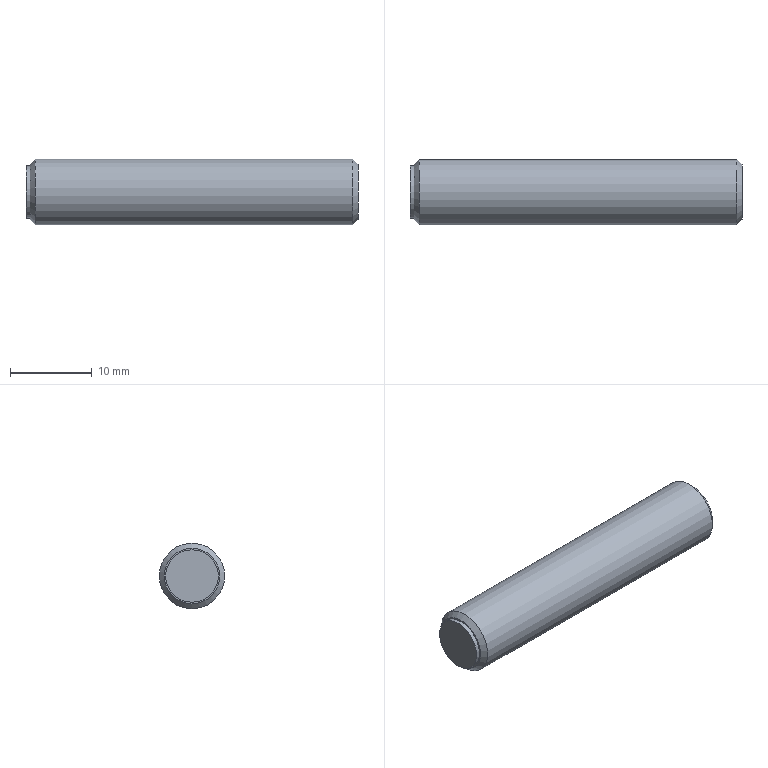Part | NX | features BREP 1 | 1 solid | 7 faces | box 40.5 x 8 x 8 mm | volume 2018 mm3 | plane 3 | cylinder 2 | cone 2 | commonest cylinder face diameters 6.4 x1 8 x1
STEP:
#1=CARTESIAN_POINT('',(1.113,0.,4.));
#2=VERTEX_POINT('',#1);
#3=CARTESIAN_POINT('',(1.113,0.,0.));
#4=DIRECTION('',(1.,0.,0.));
#5=DIRECTION('',(0.,0.,1.));
#6=AXIS2_PLACEMENT_3D('',#3,#4,#5);
#7=CIRCLE('',#6,4.);
#8=EDGE_CURVE('',#2,#2,#7,.T.);
#9=ORIENTED_EDGE('',*,*,#8,.T.);
#10=EDGE_LOOP('',(#9));
#11=FACE_BOUND('',#10,.T.);
#12=CARTESIAN_POINT('',(39.886,0.,4.));
#13=VERTEX_POINT('',#12);
#14=CARTESIAN_POINT('',(39.886,0.,0.));
#15=DIRECTION('',(-1.,0.,0.));
#16=DIRECTION('',(0.,0.,1.));
#17=AXIS2_PLACEMENT_3D('',#14,#15,#16);
#18=CIRCLE('',#17,4.);
#19=EDGE_CURVE('',#13,#13,#18,.T.);
#20=ORIENTED_EDGE('',*,*,#19,.T.);
#21=EDGE_LOOP('',(#20));
#22=FACE_BOUND('',#21,.T.);
#23=CARTESIAN_POINT('',(40.5,0.,0.));
#24=DIRECTION('',(-1.,0.,0.));
#25=DIRECTION('',(0.,0.,-1.));
#26=AXIS2_PLACEMENT_3D('',#23,#24,#25);
#27=CYLINDRICAL_SURFACE('',#26,4.);
#28=ADVANCED_FACE('',(#11,#22),#27,.T.);
#29=CARTESIAN_POINT('',(0.5,0.,-3.386));
#30=VERTEX_POINT('',#29);
#31=CARTESIAN_POINT('',(0.5,0.,0.));
#32=DIRECTION('',(1.,0.,0.));
#33=DIRECTION('',(0.,0.,-1.));
#34=AXIS2_PLACEMENT_3D('',#31,#32,#33);
#35=CIRCLE('',#34,3.386);
#36=EDGE_CURVE('',#30,#30,#35,.T.);
#37=ORIENTED_EDGE('',*,*,#36,.T.);
#38=EDGE_LOOP('',(#37));
#39=FACE_BOUND('',#38,.T.);
#40=ORIENTED_EDGE('',*,*,#8,.F.);
#41=EDGE_LOOP('',(#40));
#42=FACE_BOUND('',#41,.T.);
#43=CARTESIAN_POINT('',(1.113,0.,0.));
#44=DIRECTION('',(1.,0.,0.));
#45=DIRECTION('',(0.,0.,1.));
#46=AXIS2_PLACEMENT_3D('',#43,#44,#45);
#47=CONICAL_SURFACE('',#46,4.,0.7854);
#48=ADVANCED_FACE('',(#39,#42),#47,.T.);
#49=CARTESIAN_POINT('',(40.5,0.,3.387));
#50=VERTEX_POINT('',#49);
#51=CARTESIAN_POINT('',(40.5,0.,0.));
#52=DIRECTION('',(-1.,0.,0.));
#53=DIRECTION('',(0.,0.,1.));
#54=AXIS2_PLACEMENT_3D('',#51,#52,#53);
#55=CIRCLE('',#54,3.387);
#56=EDGE_CURVE('',#50,#50,#55,.T.);
#57=ORIENTED_EDGE('',*,*,#56,.T.);
#58=EDGE_LOOP('',(#57));
#59=FACE_BOUND('',#58,.T.);
#60=ORIENTED_EDGE('',*,*,#19,.F.);
#61=EDGE_LOOP('',(#60));
#62=FACE_BOUND('',#61,.T.);
#63=CARTESIAN_POINT('',(39.887,0.,0.));
#64=DIRECTION('',(-1.,0.,0.));
#65=DIRECTION('',(0.,0.,-1.));
#66=AXIS2_PLACEMENT_3D('',#63,#64,#65);
#67=CONICAL_SURFACE('',#66,4.,0.7854);
#68=ADVANCED_FACE('',(#59,#62),#67,.T.);
#69=ORIENTED_EDGE('',*,*,#36,.F.);
#70=EDGE_LOOP('',(#69));
#71=FACE_BOUND('',#70,.T.);
#72=CARTESIAN_POINT('',(0.5,0.,3.2));
#73=VERTEX_POINT('',#72);
#74=CARTESIAN_POINT('',(0.5,0.,0.));
#75=DIRECTION('',(-1.,0.,0.));
#76=DIRECTION('',(0.,0.,1.));
#77=AXIS2_PLACEMENT_3D('',#74,#75,#76);
#78=CIRCLE('',#77,3.2);
#79=EDGE_CURVE('',#73,#73,#78,.T.);
#80=ORIENTED_EDGE('',*,*,#79,.F.);
#81=EDGE_LOOP('',(#80));
#82=FACE_BOUND('',#81,.T.);
#83=CARTESIAN_POINT('',(0.5,0.,0.));
#84=DIRECTION('',(1.,0.,0.));
#85=DIRECTION('',(0.,0.,1.));
#86=AXIS2_PLACEMENT_3D('',#83,#84,#85);
#87=PLANE('',#86);
#88=ADVANCED_FACE('',(#71,#82),#87,.F.);
#89=ORIENTED_EDGE('',*,*,#56,.F.);
#90=EDGE_LOOP('',(#89));
#91=FACE_BOUND('',#90,.T.);
#92=CARTESIAN_POINT('',(40.5,3.386,0.));
#93=DIRECTION('',(-1.,0.,0.));
#94=DIRECTION('',(0.,0.,-1.));
#95=AXIS2_PLACEMENT_3D('',#92,#93,#94);
#96=PLANE('',#95);
#97=ADVANCED_FACE('',(#91),#96,.F.);
#98=ORIENTED_EDGE('',*,*,#79,.T.);
#99=EDGE_LOOP('',(#98));
#100=FACE_BOUND('',#99,.T.);
#101=CARTESIAN_POINT('',(0.,0.,3.2));
#102=VERTEX_POINT('',#101);
#103=CARTESIAN_POINT('',(0.,0.,0.));
#104=DIRECTION('',(1.,0.,0.));
#105=DIRECTION('',(0.,0.,1.));
#106=AXIS2_PLACEMENT_3D('',#103,#104,#105);
#107=CIRCLE('',#106,3.2);
#108=EDGE_CURVE('',#102,#102,#107,.T.);
#109=ORIENTED_EDGE('',*,*,#108,.T.);
#110=EDGE_LOOP('',(#109));
#111=FACE_BOUND('',#110,.T.);
#112=CARTESIAN_POINT('',(0.5,0.,0.));
#113=DIRECTION('',(-1.,0.,0.));
#114=DIRECTION('',(0.,0.,-1.));
#115=AXIS2_PLACEMENT_3D('',#112,#113,#114);
#116=CYLINDRICAL_SURFACE('',#115,3.2);
#117=ADVANCED_FACE('',(#100,#111),#116,.T.);
#118=ORIENTED_EDGE('',*,*,#108,.F.);
#119=EDGE_LOOP('',(#118));
#120=FACE_BOUND('',#119,.T.);
#121=CARTESIAN_POINT('',(0.,0.,0.));
#122=DIRECTION('',(1.,0.,0.));
#123=DIRECTION('',(0.,0.,1.));
#124=AXIS2_PLACEMENT_3D('',#121,#122,#123);
#125=PLANE('',#124);
#126=ADVANCED_FACE('',(#120),#125,.F.);
#127=CLOSED_SHELL('',(#28,#48,#68,#88,#97,#117,#126));
#128=MANIFOLD_SOLID_BREP('',#127);
#129=(LENGTH_UNIT()NAMED_UNIT(*)SI_UNIT(.MILLI.,.METRE.));
#130=UNCERTAINTY_MEASURE_WITH_UNIT(LENGTH_MEASURE(0.00001),#129,'','');
#131=(NAMED_UNIT(*)PLANE_ANGLE_UNIT()SI_UNIT($,.RADIAN.));
#132=(NAMED_UNIT(*)SI_UNIT($,.STERADIAN.)SOLID_ANGLE_UNIT());
#133=(GEOMETRIC_REPRESENTATION_CONTEXT(3)GLOBAL_UNCERTAINTY_ASSIGNED_CONTEXT((#130))GLOBAL_UNIT_ASSIGNED_CONTEXT((#129,#131,#132))REPRESENTATION_CONTEXT('',''));
#134=ADVANCED_BREP_SHAPE_REPRESENTATION('',(#128),#133);